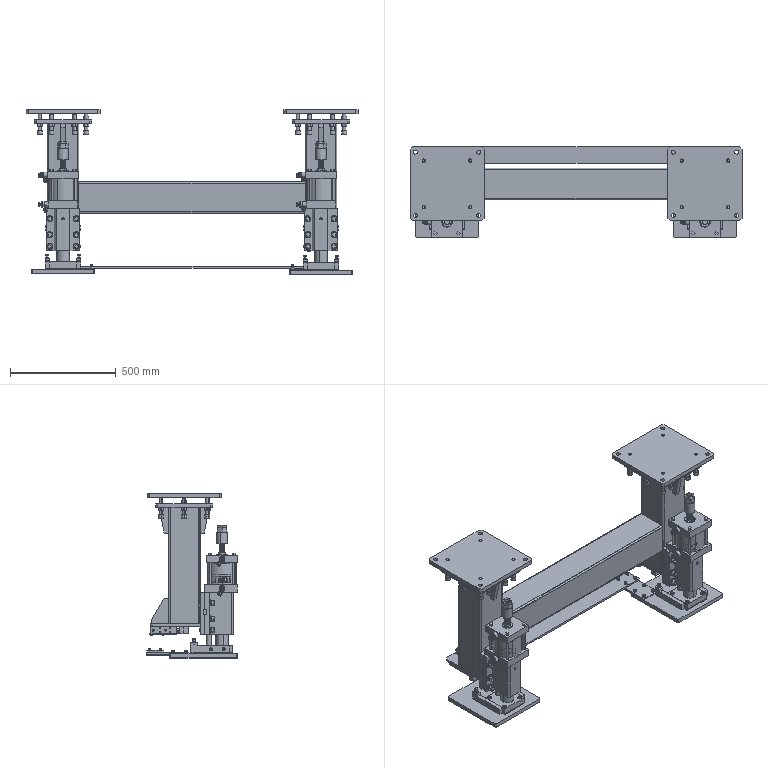Part | SolidWorks | features ReferencePattern 33, LocalLPattern 4, CompositeCurve 3 | 218 solids | 6048 faces | volume 32750415 mm3 | plane 2244 | cylinder 2208 | cone 1138 | torus 352 | spline 90 | sphere 16 | commonest cylinder face diameters 27 x218 12 x174 16 x160 10 x110 14 x88 8 x72